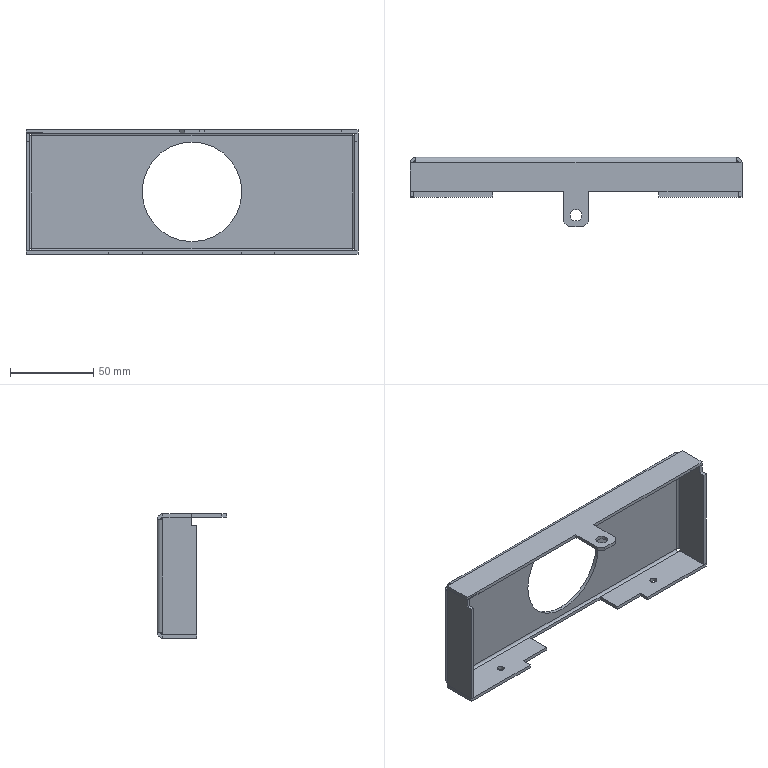Part | STEP file | Slide plate seat | 1 solid | 76 faces | box 200 x 42 x 75 mm | volume 42985 mm3 | plane 60 | cylinder 16 | commonest cylinder face diameters 7 x6 3 x4 4.2 x4 60 x2